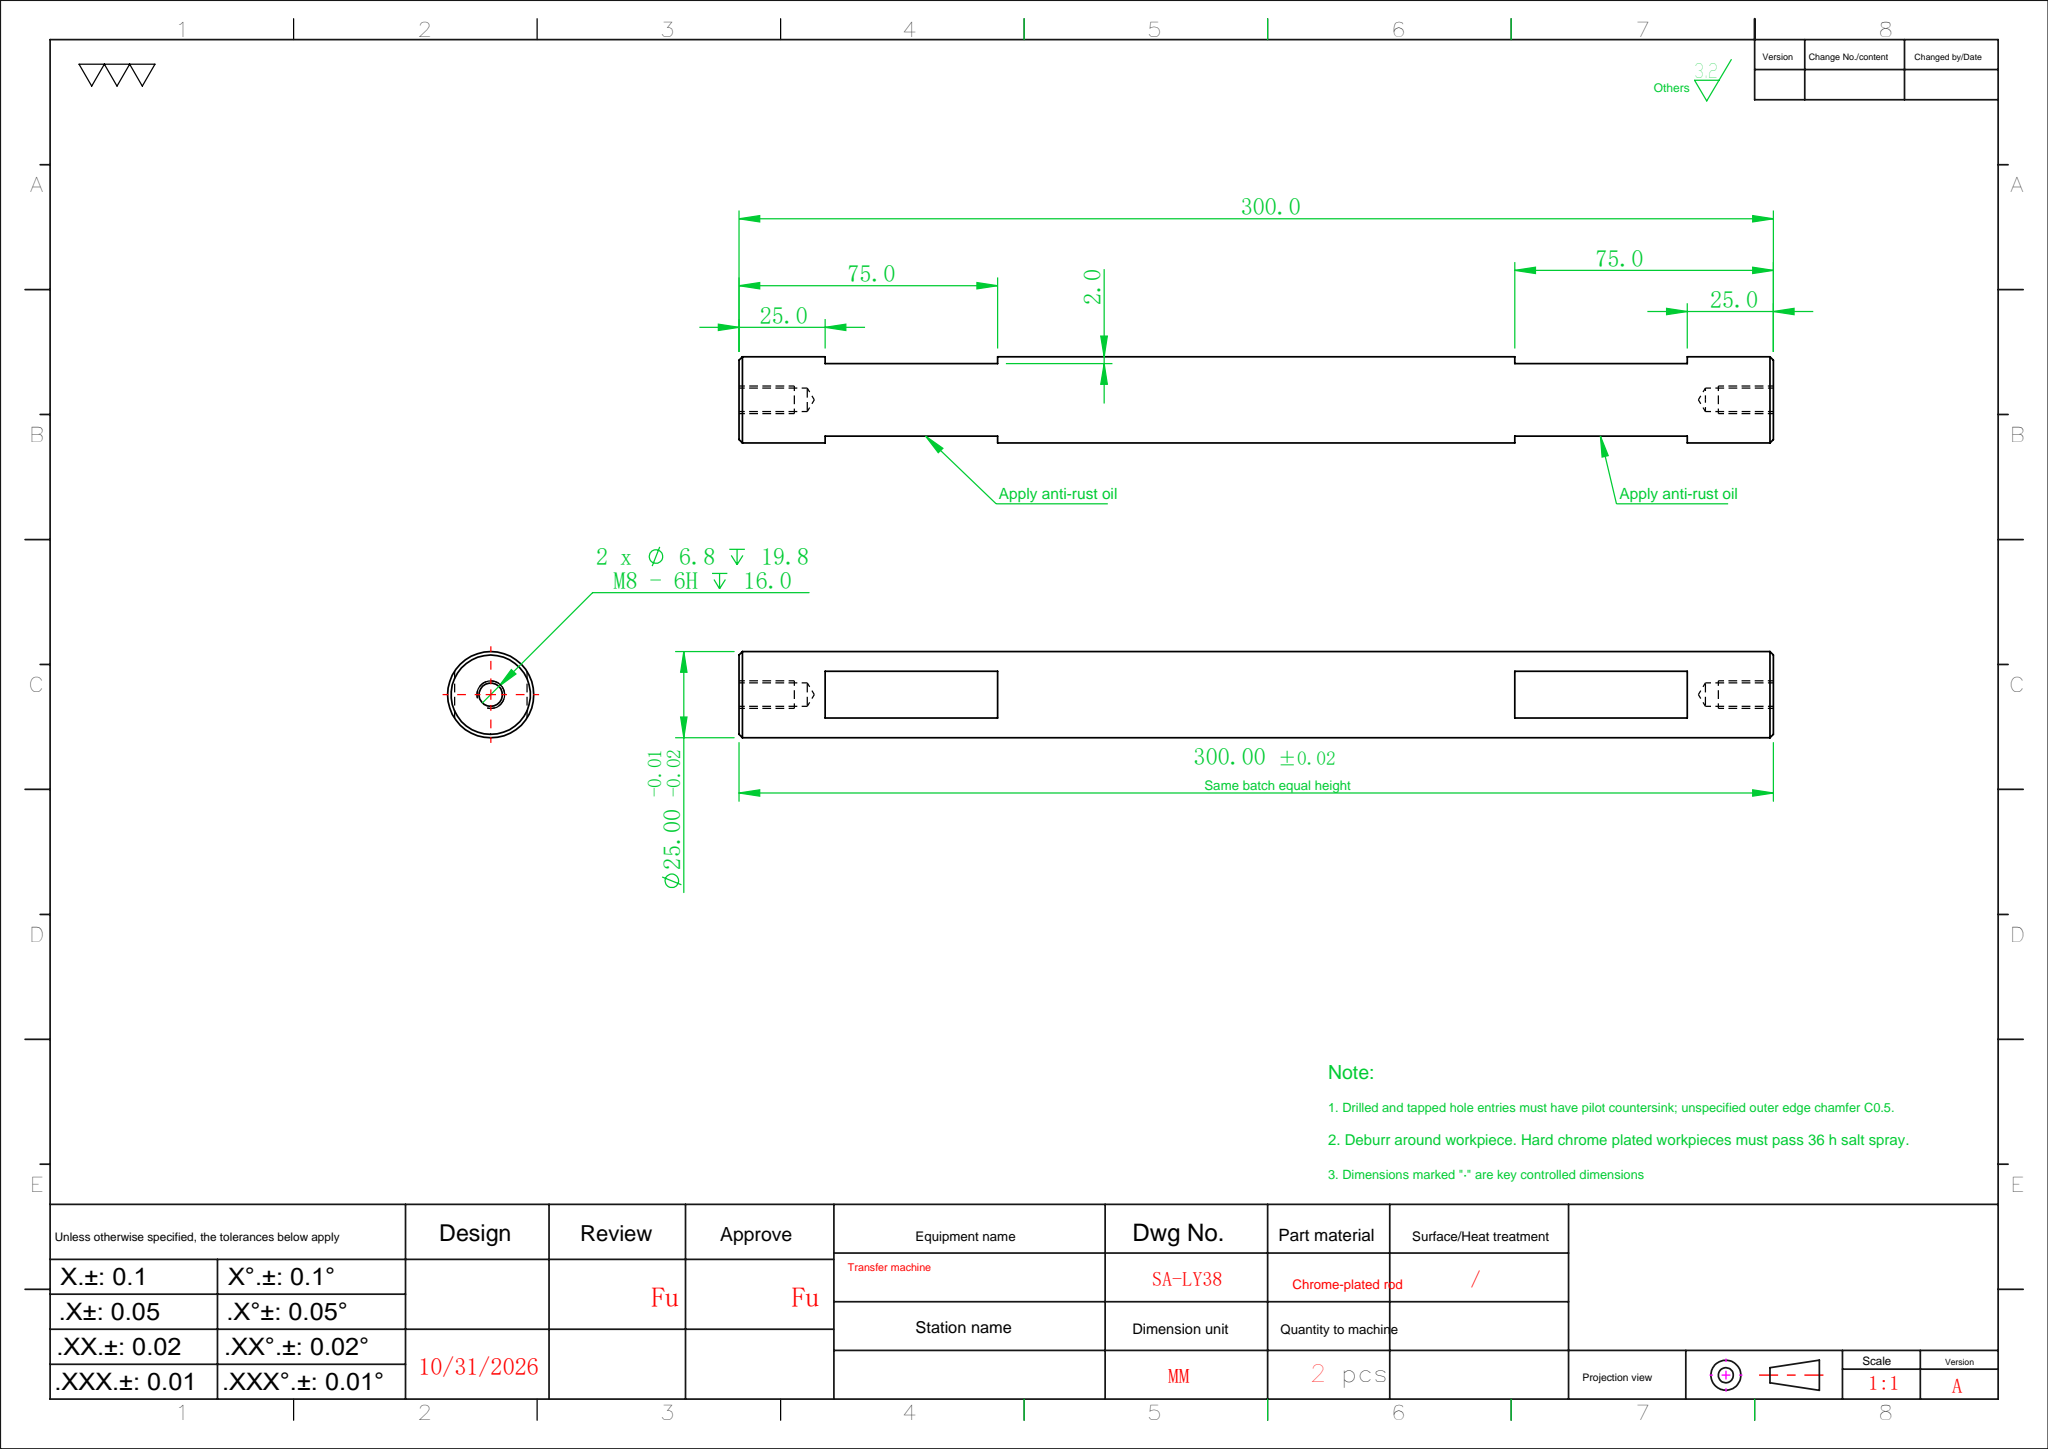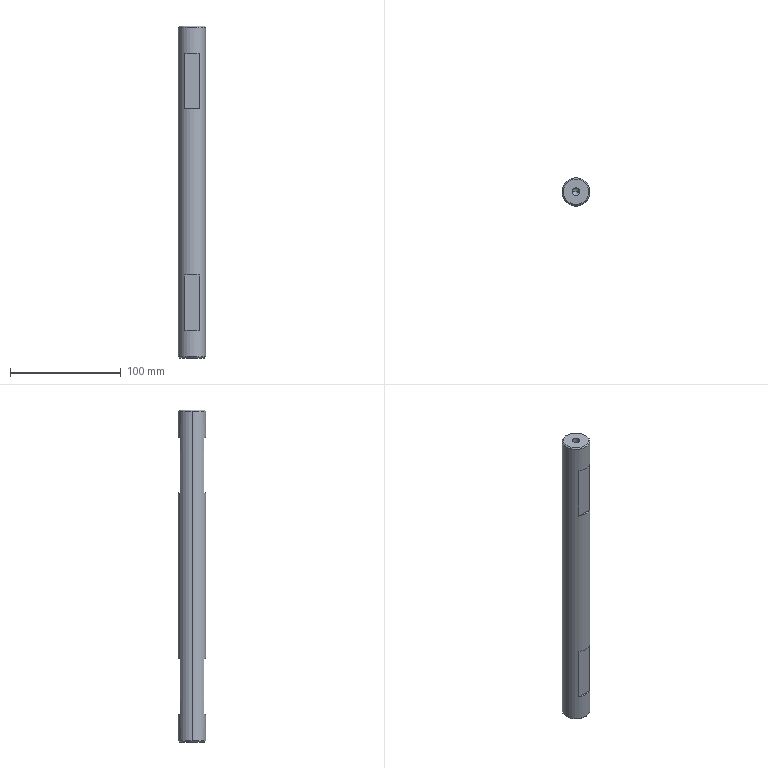Part | SolidWorks | features Chamfer 1, Extrusion 1, HoleWzd 1, ICE 1, MirrorPattern 1 | 1 solid | 28 faces | box 25 x 25 x 300 mm | volume 142022 mm3 | plane 14 | cone 8 | cylinder 6 | commonest cylinder face diameters 6.8 x4 25 x2
STEP:
#1=CARTESIAN_POINT('',(-3.4,0.,130.25));
#2=VERTEX_POINT('',#1);
#3=CARTESIAN_POINT('',(3.4,0.,130.25));
#4=VERTEX_POINT('',#3);
#5=CARTESIAN_POINT('',(0.,0.,130.25));
#6=DIRECTION('',(0.,0.,1.));
#7=DIRECTION('',(1.,0.,0.));
#8=AXIS2_PLACEMENT_3D('',#5,#6,#7);
#9=CIRCLE('',#8,3.4);
#10=EDGE_CURVE('',#2,#4,#9,.T.);
#11=ORIENTED_EDGE('',*,*,#10,.F.);
#12=CARTESIAN_POINT('',(-3.4,0.,150.));
#13=VERTEX_POINT('',#12);
#14=CARTESIAN_POINT('',(-3.4,0.,150.));
#15=DIRECTION('',(0.,0.,1.));
#16=VECTOR('',#15,1000.);
#17=LINE('',#14,#16);
#18=EDGE_CURVE('',#2,#13,#17,.T.);
#19=ORIENTED_EDGE('',*,*,#18,.T.);
#20=CARTESIAN_POINT('',(3.4,0.,150.));
#21=VERTEX_POINT('',#20);
#22=CARTESIAN_POINT('',(0.,0.,150.));
#23=DIRECTION('',(0.,0.,1.));
#24=DIRECTION('',(1.,0.,0.));
#25=AXIS2_PLACEMENT_3D('',#22,#23,#24);
#26=CIRCLE('',#25,3.4);
#27=EDGE_CURVE('',#13,#21,#26,.T.);
#28=ORIENTED_EDGE('',*,*,#27,.T.);
#29=CARTESIAN_POINT('',(3.4,0.,150.));
#30=DIRECTION('',(0.,0.,1.));
#31=VECTOR('',#30,1000.);
#32=LINE('',#29,#31);
#33=EDGE_CURVE('',#4,#21,#32,.T.);
#34=ORIENTED_EDGE('',*,*,#33,.F.);
#35=EDGE_LOOP('',(#11,#19,#28,#34));
#36=FACE_OUTER_BOUND('',#35,.T.);
#37=CARTESIAN_POINT('',(0.,0.,150.));
#38=DIRECTION('',(0.,0.,1.));
#39=DIRECTION('',(1.,0.,0.));
#40=AXIS2_PLACEMENT_3D('',#37,#38,#39);
#41=CYLINDRICAL_SURFACE('',#40,3.4);
#42=ADVANCED_FACE('',(#36),#41,.F.);
#43=CARTESIAN_POINT('',(0.,0.,128.207));
#44=VERTEX_POINT('',#43);
#45=CARTESIAN_POINT('',(3.4,0.,130.25));
#46=DIRECTION('',(0.8572,0.,0.515));
#47=VECTOR('',#46,1000.);
#48=LINE('',#45,#47);
#49=EDGE_CURVE('',#44,#4,#48,.T.);
#50=ORIENTED_EDGE('',*,*,#49,.F.);
#51=CARTESIAN_POINT('',(-3.4,0.,130.25));
#52=DIRECTION('',(-0.8572,0.,0.515));
#53=VECTOR('',#52,1000.);
#54=LINE('',#51,#53);
#55=EDGE_CURVE('',#44,#2,#54,.T.);
#56=ORIENTED_EDGE('',*,*,#55,.T.);
#57=ORIENTED_EDGE('',*,*,#10,.T.);
#58=EDGE_LOOP('',(#50,#56,#57));
#59=FACE_OUTER_BOUND('',#58,.T.);
#60=CARTESIAN_POINT('',(0.,0.,130.25));
#61=DIRECTION('',(0.,0.,1.));
#62=DIRECTION('',(1.,0.,0.));
#63=AXIS2_PLACEMENT_3D('',#60,#61,#62);
#64=CONICAL_SURFACE('',#63,3.4,1.03);
#65=ADVANCED_FACE('',(#59),#64,.F.);
#66=CARTESIAN_POINT('',(3.4,0.,-130.25));
#67=VERTEX_POINT('',#66);
#68=CARTESIAN_POINT('',(-3.4,0.,-130.25));
#69=VERTEX_POINT('',#68);
#70=CARTESIAN_POINT('',(0.,0.,-130.25));
#71=DIRECTION('',(0.,0.,-1.));
#72=DIRECTION('',(-1.,0.,0.));
#73=AXIS2_PLACEMENT_3D('',#70,#71,#72);
#74=CIRCLE('',#73,3.4);
#75=EDGE_CURVE('',#67,#69,#74,.T.);
#76=ORIENTED_EDGE('',*,*,#75,.F.);
#77=CARTESIAN_POINT('',(3.4,0.,-150.));
#78=VERTEX_POINT('',#77);
#79=CARTESIAN_POINT('',(3.4,0.,-150.));
#80=DIRECTION('',(0.,0.,-1.));
#81=VECTOR('',#80,1000.);
#82=LINE('',#79,#81);
#83=EDGE_CURVE('',#67,#78,#82,.T.);
#84=ORIENTED_EDGE('',*,*,#83,.T.);
#85=CARTESIAN_POINT('',(-3.4,0.,-150.));
#86=VERTEX_POINT('',#85);
#87=CARTESIAN_POINT('',(0.,0.,-150.));
#88=DIRECTION('',(0.,0.,-1.));
#89=DIRECTION('',(-1.,0.,0.));
#90=AXIS2_PLACEMENT_3D('',#87,#88,#89);
#91=CIRCLE('',#90,3.4);
#92=EDGE_CURVE('',#78,#86,#91,.T.);
#93=ORIENTED_EDGE('',*,*,#92,.T.);
#94=CARTESIAN_POINT('',(-3.4,0.,-150.));
#95=DIRECTION('',(0.,0.,-1.));
#96=VECTOR('',#95,1000.);
#97=LINE('',#94,#96);
#98=EDGE_CURVE('',#69,#86,#97,.T.);
#99=ORIENTED_EDGE('',*,*,#98,.F.);
#100=EDGE_LOOP('',(#76,#84,#93,#99));
#101=FACE_OUTER_BOUND('',#100,.T.);
#102=CARTESIAN_POINT('',(0.,0.,-150.));
#103=DIRECTION('',(0.,0.,-1.));
#104=DIRECTION('',(-1.,0.,0.));
#105=AXIS2_PLACEMENT_3D('',#102,#103,#104);
#106=CYLINDRICAL_SURFACE('',#105,3.4);
#107=ADVANCED_FACE('',(#101),#106,.F.);
#108=CARTESIAN_POINT('',(0.,0.,-128.207));
#109=VERTEX_POINT('',#108);
#110=CARTESIAN_POINT('',(-3.4,0.,-130.25));
#111=DIRECTION('',(-0.8572,0.,-0.515));
#112=VECTOR('',#111,1000.);
#113=LINE('',#110,#112);
#114=EDGE_CURVE('',#109,#69,#113,.T.);
#115=ORIENTED_EDGE('',*,*,#114,.F.);
#116=CARTESIAN_POINT('',(3.4,0.,-130.25));
#117=DIRECTION('',(0.8572,0.,-0.515));
#118=VECTOR('',#117,1000.);
#119=LINE('',#116,#118);
#120=EDGE_CURVE('',#109,#67,#119,.T.);
#121=ORIENTED_EDGE('',*,*,#120,.T.);
#122=ORIENTED_EDGE('',*,*,#75,.T.);
#123=EDGE_LOOP('',(#115,#121,#122));
#124=FACE_OUTER_BOUND('',#123,.T.);
#125=CARTESIAN_POINT('',(0.,0.,-130.25));
#126=DIRECTION('',(0.,0.,-1.));
#127=DIRECTION('',(-1.,0.,0.));
#128=AXIS2_PLACEMENT_3D('',#125,#126,#127);
#129=CONICAL_SURFACE('',#128,3.4,1.03);
#130=ADVANCED_FACE('',(#124),#129,.F.);
#131=CARTESIAN_POINT('',(-11.5,0.,-150.));
#132=VERTEX_POINT('',#131);
#133=CARTESIAN_POINT('',(11.5,0.,-150.));
#134=VERTEX_POINT('',#133);
#135=CARTESIAN_POINT('',(0.,0.,-150.));
#136=DIRECTION('',(0.,0.,-1.));
#137=DIRECTION('',(1.,0.,0.));
#138=AXIS2_PLACEMENT_3D('',#135,#136,#137);
#139=CIRCLE('',#138,11.5);
#140=EDGE_CURVE('',#132,#134,#139,.T.);
#141=ORIENTED_EDGE('',*,*,#140,.F.);
#142=CARTESIAN_POINT('',(-12.5,0.,-149.));
#143=VERTEX_POINT('',#142);
#144=CARTESIAN_POINT('',(-12.5,0.,-149.));
#145=DIRECTION('',(-0.7071,0.,0.7071));
#146=VECTOR('',#145,1000.);
#147=LINE('',#144,#146);
#148=EDGE_CURVE('',#132,#143,#147,.T.);
#149=ORIENTED_EDGE('',*,*,#148,.T.);
#150=CARTESIAN_POINT('',(12.5,0.,-149.));
#151=VERTEX_POINT('',#150);
#152=CARTESIAN_POINT('',(0.,0.,-149.));
#153=DIRECTION('',(0.,0.,1.));
#154=DIRECTION('',(1.,0.,0.));
#155=AXIS2_PLACEMENT_3D('',#152,#153,#154);
#156=CIRCLE('',#155,12.5);
#157=EDGE_CURVE('',#151,#143,#156,.T.);
#158=ORIENTED_EDGE('',*,*,#157,.F.);
#159=CARTESIAN_POINT('',(12.5,0.,-149.));
#160=DIRECTION('',(0.7071,0.,0.7071));
#161=VECTOR('',#160,1000.);
#162=LINE('',#159,#161);
#163=EDGE_CURVE('',#134,#151,#162,.T.);
#164=ORIENTED_EDGE('',*,*,#163,.F.);
#165=EDGE_LOOP('',(#141,#149,#158,#164));
#166=FACE_OUTER_BOUND('',#165,.T.);
#167=CARTESIAN_POINT('',(0.,0.,-149.));
#168=DIRECTION('',(0.,0.,1.));
#169=DIRECTION('',(1.,0.,0.));
#170=AXIS2_PLACEMENT_3D('',#167,#168,#169);
#171=CONICAL_SURFACE('',#170,12.5,0.7854);
#172=ADVANCED_FACE('',(#166),#171,.T.);
#173=CARTESIAN_POINT('',(11.5,0.,150.));
#174=VERTEX_POINT('',#173);
#175=CARTESIAN_POINT('',(-11.5,0.,150.));
#176=VERTEX_POINT('',#175);
#177=CARTESIAN_POINT('',(0.,0.,150.));
#178=DIRECTION('',(0.,0.,1.));
#179=DIRECTION('',(1.,0.,0.));
#180=AXIS2_PLACEMENT_3D('',#177,#178,#179);
#181=CIRCLE('',#180,11.5);
#182=EDGE_CURVE('',#174,#176,#181,.T.);
#183=ORIENTED_EDGE('',*,*,#182,.F.);
#184=CARTESIAN_POINT('',(12.5,0.,149.));
#185=VERTEX_POINT('',#184);
#186=CARTESIAN_POINT('',(11.5,0.,150.));
#187=DIRECTION('',(0.7071,0.,-0.7071));
#188=VECTOR('',#187,1000.);
#189=LINE('',#186,#188);
#190=EDGE_CURVE('',#174,#185,#189,.T.);
#191=ORIENTED_EDGE('',*,*,#190,.T.);
#192=CARTESIAN_POINT('',(-12.5,0.,149.));
#193=VERTEX_POINT('',#192);
#194=CARTESIAN_POINT('',(0.,0.,149.));
#195=DIRECTION('',(0.,0.,-1.));
#196=DIRECTION('',(1.,0.,0.));
#197=AXIS2_PLACEMENT_3D('',#194,#195,#196);
#198=CIRCLE('',#197,12.5);
#199=EDGE_CURVE('',#193,#185,#198,.T.);
#200=ORIENTED_EDGE('',*,*,#199,.F.);
#201=CARTESIAN_POINT('',(-11.5,0.,150.));
#202=DIRECTION('',(-0.7071,0.,-0.7071));
#203=VECTOR('',#202,1000.);
#204=LINE('',#201,#203);
#205=EDGE_CURVE('',#176,#193,#204,.T.);
#206=ORIENTED_EDGE('',*,*,#205,.F.);
#207=EDGE_LOOP('',(#183,#191,#200,#206));
#208=FACE_OUTER_BOUND('',#207,.T.);
#209=CARTESIAN_POINT('',(0.,0.,150.));
#210=DIRECTION('',(0.,0.,-1.));
#211=DIRECTION('',(-1.,0.,0.));
#212=AXIS2_PLACEMENT_3D('',#209,#210,#211);
#213=CONICAL_SURFACE('',#212,11.5,0.7854);
#214=ADVANCED_FACE('',(#208),#213,.T.);
#215=CARTESIAN_POINT('',(6.782,10.5,125.));
#216=VERTEX_POINT('',#215);
#217=CARTESIAN_POINT('',(-6.782,10.5,125.));
#218=VERTEX_POINT('',#217);
#219=CARTESIAN_POINT('',(0.,0.,125.));
#220=DIRECTION('',(0.,0.,1.));
#221=DIRECTION('',(1.,0.,0.));
#222=AXIS2_PLACEMENT_3D('',#219,#220,#221);
#223=CIRCLE('',#222,12.5);
#224=EDGE_CURVE('',#216,#218,#223,.T.);
#225=ORIENTED_EDGE('',*,*,#224,.T.);
#226=CARTESIAN_POINT('',(-6.782,10.5,75.));
#227=VERTEX_POINT('',#226);
#228=CARTESIAN_POINT('',(-6.782,10.5,150.));
#229=DIRECTION('',(0.,0.,-1.));
#230=VECTOR('',#229,1000.);
#231=LINE('',#228,#230);
#232=EDGE_CURVE('',#218,#227,#231,.T.);
#233=ORIENTED_EDGE('',*,*,#232,.T.);
#234=CARTESIAN_POINT('',(6.782,10.5,75.));
#235=VERTEX_POINT('',#234);
#236=CARTESIAN_POINT('',(0.,0.,75.));
#237=DIRECTION('',(0.,0.,-1.));
#238=DIRECTION('',(-1.,0.,0.));
#239=AXIS2_PLACEMENT_3D('',#236,#237,#238);
#240=CIRCLE('',#239,12.5);
#241=EDGE_CURVE('',#227,#235,#240,.T.);
#242=ORIENTED_EDGE('',*,*,#241,.T.);
#243=CARTESIAN_POINT('',(6.782,10.5,150.));
#244=DIRECTION('',(0.,0.,1.));
#245=VECTOR('',#244,1000.);
#246=LINE('',#243,#245);
#247=EDGE_CURVE('',#235,#216,#246,.T.);
#248=ORIENTED_EDGE('',*,*,#247,.T.);
#249=EDGE_LOOP('',(#225,#233,#242,#248));
#250=FACE_BOUND('',#249,.T.);
#251=CARTESIAN_POINT('',(-6.782,10.5,-75.));
#252=VERTEX_POINT('',#251);
#253=CARTESIAN_POINT('',(-6.782,10.5,-125.));
#254=VERTEX_POINT('',#253);
#255=CARTESIAN_POINT('',(-6.782,10.5,150.));
#256=DIRECTION('',(0.,0.,-1.));
#257=VECTOR('',#256,1000.);
#258=LINE('',#255,#257);
#259=EDGE_CURVE('',#252,#254,#258,.T.);
#260=ORIENTED_EDGE('',*,*,#259,.T.);
#261=CARTESIAN_POINT('',(6.782,10.5,-125.));
#262=VERTEX_POINT('',#261);
#263=CARTESIAN_POINT('',(0.,0.,-125.));
#264=DIRECTION('',(0.,0.,-1.));
#265=DIRECTION('',(-1.,0.,0.));
#266=AXIS2_PLACEMENT_3D('',#263,#264,#265);
#267=CIRCLE('',#266,12.5);
#268=EDGE_CURVE('',#254,#262,#267,.T.);
#269=ORIENTED_EDGE('',*,*,#268,.T.);
#270=CARTESIAN_POINT('',(6.782,10.5,-75.));
#271=VERTEX_POINT('',#270);
#272=CARTESIAN_POINT('',(6.782,10.5,150.));
#273=DIRECTION('',(0.,0.,1.));
#274=VECTOR('',#273,1000.);
#275=LINE('',#272,#274);
#276=EDGE_CURVE('',#262,#271,#275,.T.);
#277=ORIENTED_EDGE('',*,*,#276,.T.);
#278=CARTESIAN_POINT('',(0.,0.,-75.));
#279=DIRECTION('',(0.,0.,1.));
#280=DIRECTION('',(1.,0.,0.));
#281=AXIS2_PLACEMENT_3D('',#278,#279,#280);
#282=CIRCLE('',#281,12.5);
#283=EDGE_CURVE('',#271,#252,#282,.T.);
#284=ORIENTED_EDGE('',*,*,#283,.T.);
#285=EDGE_LOOP('',(#260,#269,#277,#284));
#286=FACE_BOUND('',#285,.T.);
#287=ORIENTED_EDGE('',*,*,#199,.T.);
#288=CARTESIAN_POINT('',(12.5,0.,150.));
#289=DIRECTION('',(0.,0.,-1.));
#290=VECTOR('',#289,1000.);
#291=LINE('',#288,#290);
#292=EDGE_CURVE('',#185,#151,#291,.T.);
#293=ORIENTED_EDGE('',*,*,#292,.T.);
#294=ORIENTED_EDGE('',*,*,#157,.T.);
#295=CARTESIAN_POINT('',(-12.5,0.,150.));
#296=DIRECTION('',(0.,0.,-1.));
#297=VECTOR('',#296,1000.);
#298=LINE('',#295,#297);
#299=EDGE_CURVE('',#193,#143,#298,.T.);
#300=ORIENTED_EDGE('',*,*,#299,.F.);
#301=EDGE_LOOP('',(#287,#293,#294,#300));
#302=FACE_OUTER_BOUND('',#301,.T.);
#303=CARTESIAN_POINT('',(0.,0.,150.));
#304=DIRECTION('',(0.,0.,-1.));
#305=DIRECTION('',(-1.,0.,0.));
#306=AXIS2_PLACEMENT_3D('',#303,#304,#305);
#307=CYLINDRICAL_SURFACE('',#306,12.5);
#308=ADVANCED_FACE('',(#250,#286,#302),#307,.T.);
#309=ORIENTED_EDGE('',*,*,#292,.F.);
#310=CARTESIAN_POINT('',(0.,0.,149.));
#311=DIRECTION('',(0.,0.,-1.));
#312=DIRECTION('',(1.,0.,0.));
#313=AXIS2_PLACEMENT_3D('',#310,#311,#312);
#314=CIRCLE('',#313,12.5);
#315=EDGE_CURVE('',#185,#193,#314,.T.);
#316=ORIENTED_EDGE('',*,*,#315,.T.);
#317=ORIENTED_EDGE('',*,*,#299,.T.);
#318=CARTESIAN_POINT('',(0.,0.,-149.));
#319=DIRECTION('',(0.,0.,1.));
#320=DIRECTION('',(1.,0.,0.));
#321=AXIS2_PLACEMENT_3D('',#318,#319,#320);
#322=CIRCLE('',#321,12.5);
#323=EDGE_CURVE('',#143,#151,#322,.T.);
#324=ORIENTED_EDGE('',*,*,#323,.T.);
#325=EDGE_LOOP('',(#309,#316,#317,#324));
#326=FACE_OUTER_BOUND('',#325,.T.);
#327=CARTESIAN_POINT('',(-6.782,-10.5,-75.));
#328=VERTEX_POINT('',#327);
#329=CARTESIAN_POINT('',(6.782,-10.5,-75.));
#330=VERTEX_POINT('',#329);
#331=CARTESIAN_POINT('',(0.,0.,-75.));
#332=DIRECTION('',(0.,0.,1.));
#333=DIRECTION('',(1.,0.,0.));
#334=AXIS2_PLACEMENT_3D('',#331,#332,#333);
#335=CIRCLE('',#334,12.5);
#336=EDGE_CURVE('',#328,#330,#335,.T.);
#337=ORIENTED_EDGE('',*,*,#336,.T.);
#338=CARTESIAN_POINT('',(6.782,-10.5,-125.));
#339=VERTEX_POINT('',#338);
#340=CARTESIAN_POINT('',(6.782,-10.5,150.));
#341=DIRECTION('',(0.,0.,-1.));
#342=VECTOR('',#341,1000.);
#343=LINE('',#340,#342);
#344=EDGE_CURVE('',#330,#339,#343,.T.);
#345=ORIENTED_EDGE('',*,*,#344,.T.);
#346=CARTESIAN_POINT('',(-6.782,-10.5,-125.));
#347=VERTEX_POINT('',#346);
#348=CARTESIAN_POINT('',(0.,0.,-125.));
#349=DIRECTION('',(0.,0.,-1.));
#350=DIRECTION('',(-1.,0.,0.));
#351=AXIS2_PLACEMENT_3D('',#348,#349,#350);
#352=CIRCLE('',#351,12.5);
#353=EDGE_CURVE('',#339,#347,#352,.T.);
#354=ORIENTED_EDGE('',*,*,#353,.T.);
#355=CARTESIAN_POINT('',(-6.782,-10.5,150.));
#356=DIRECTION('',(0.,0.,1.));
#357=VECTOR('',#356,1000.);
#358=LINE('',#355,#357);
#359=EDGE_CURVE('',#347,#328,#358,.T.);
#360=ORIENTED_EDGE('',*,*,#359,.T.);
#361=EDGE_LOOP('',(#337,#345,#354,#360));
#362=FACE_BOUND('',#361,.T.);
#363=CARTESIAN_POINT('',(-6.782,-10.5,75.));
#364=VERTEX_POINT('',#363);
#365=CARTESIAN_POINT('',(-6.782,-10.5,125.));
#366=VERTEX_POINT('',#365);
#367=CARTESIAN_POINT('',(-6.782,-10.5,150.));
#368=DIRECTION('',(0.,0.,1.));
#369=VECTOR('',#368,1000.);
#370=LINE('',#367,#369);
#371=EDGE_CURVE('',#364,#366,#370,.T.);
#372=ORIENTED_EDGE('',*,*,#371,.T.);
#373=CARTESIAN_POINT('',(6.782,-10.5,125.));
#374=VERTEX_POINT('',#373);
#375=CARTESIAN_POINT('',(0.,0.,125.));
#376=DIRECTION('',(0.,0.,1.));
#377=DIRECTION('',(1.,0.,0.));
#378=AXIS2_PLACEMENT_3D('',#375,#376,#377);
#379=CIRCLE('',#378,12.5);
#380=EDGE_CURVE('',#366,#374,#379,.T.);
#381=ORIENTED_EDGE('',*,*,#380,.T.);
#382=CARTESIAN_POINT('',(6.782,-10.5,75.));
#383=VERTEX_POINT('',#382);
#384=CARTESIAN_POINT('',(6.782,-10.5,150.));
#385=DIRECTION('',(0.,0.,-1.));
#386=VECTOR('',#385,1000.);
#387=LINE('',#384,#386);
#388=EDGE_CURVE('',#374,#383,#387,.T.);
#389=ORIENTED_EDGE('',*,*,#388,.T.);
#390=CARTESIAN_POINT('',(0.,0.,75.));
#391=DIRECTION('',(0.,0.,-1.));
#392=DIRECTION('',(-1.,0.,0.));
#393=AXIS2_PLACEMENT_3D('',#390,#391,#392);
#394=CIRCLE('',#393,12.5);
#395=EDGE_CURVE('',#383,#364,#394,.T.);
#396=ORIENTED_EDGE('',*,*,#395,.T.);
#397=EDGE_LOOP('',(#372,#381,#389,#396));
#398=FACE_BOUND('',#397,.T.);
#399=CARTESIAN_POINT('',(0.,0.,150.));
#400=DIRECTION('',(0.,0.,-1.));
#401=DIRECTION('',(-1.,0.,0.));
#402=AXIS2_PLACEMENT_3D('',#399,#400,#401);
#403=CYLINDRICAL_SURFACE('',#402,12.5);
#404=ADVANCED_FACE('',(#326,#362,#398),#403,.T.);
#405=CARTESIAN_POINT('',(0.,0.,150.));
#406=DIRECTION('',(0.,0.,1.));
#407=DIRECTION('',(1.,0.,0.));
#408=AXIS2_PLACEMENT_3D('',#405,#406,#407);
#409=CIRCLE('',#408,3.4);
#410=EDGE_CURVE('',#21,#13,#409,.T.);
#411=ORIENTED_EDGE('',*,*,#410,.F.);
#412=ORIENTED_EDGE('',*,*,#27,.F.);
#413=EDGE_LOOP('',(#411,#412));
#414=FACE_BOUND('',#413,.T.);
#415=CARTESIAN_POINT('',(0.,0.,150.));
#416=DIRECTION('',(0.,0.,1.));
#417=DIRECTION('',(1.,0.,0.));
#418=AXIS2_PLACEMENT_3D('',#415,#416,#417);
#419=CIRCLE('',#418,11.5);
#420=EDGE_CURVE('',#176,#174,#419,.T.);
#421=ORIENTED_EDGE('',*,*,#420,.T.);
#422=ORIENTED_EDGE('',*,*,#182,.T.);
#423=EDGE_LOOP('',(#421,#422));
#424=FACE_OUTER_BOUND('',#423,.T.);
#425=CARTESIAN_POINT('',(0.,0.,150.));
#426=DIRECTION('',(0.,0.,1.));
#427=DIRECTION('',(1.,0.,0.));
#428=AXIS2_PLACEMENT_3D('',#425,#426,#427);
#429=PLANE('',#428);
#430=ADVANCED_FACE('',(#414,#424),#429,.T.);
#431=CARTESIAN_POINT('',(0.,0.,-150.));
#432=DIRECTION('',(0.,0.,-1.));
#433=DIRECTION('',(-1.,0.,0.));
#434=AXIS2_PLACEMENT_3D('',#431,#432,#433);
#435=CIRCLE('',#434,3.4);
#436=EDGE_CURVE('',#86,#78,#435,.T.);
#437=ORIENTED_EDGE('',*,*,#436,.F.);
#438=ORIENTED_EDGE('',*,*,#92,.F.);
#439=EDGE_LOOP('',(#437,#438));
#440=FACE_BOUND('',#439,.T.);
#441=CARTESIAN_POINT('',(0.,0.,-150.));
#442=DIRECTION('',(0.,0.,-1.));
#443=DIRECTION('',(1.,0.,0.));
#444=AXIS2_PLACEMENT_3D('',#441,#442,#443);
#445=CIRCLE('',#444,11.5);
#446=EDGE_CURVE('',#134,#132,#445,.T.);
#447=ORIENTED_EDGE('',*,*,#446,.T.);
#448=ORIENTED_EDGE('',*,*,#140,.T.);
#449=EDGE_LOOP('',(#447,#448));
#450=FACE_OUTER_BOUND('',#449,.T.);
#451=CARTESIAN_POINT('',(0.,0.,-150.));
#452=DIRECTION('',(0.,0.,1.));
#453=DIRECTION('',(1.,0.,0.));
#454=AXIS2_PLACEMENT_3D('',#451,#452,#453);
#455=PLANE('',#454);
#456=ADVANCED_FACE('',(#440,#450),#455,.F.);
#457=CARTESIAN_POINT('',(-100.,10.5,125.));
#458=DIRECTION('',(1.,0.,0.));
#459=VECTOR('',#458,1000.);
#460=LINE('',#457,#459);
#461=EDGE_CURVE('',#218,#216,#460,.T.);
#462=ORIENTED_EDGE('',*,*,#461,.F.);
#463=ORIENTED_EDGE('',*,*,#224,.F.);
#464=EDGE_LOOP('',(#462,#463));
#465=FACE_OUTER_BOUND('',#464,.T.);
#466=CARTESIAN_POINT('',(-100.,12.5,125.));
#467=DIRECTION('',(0.,0.,1.));
#468=DIRECTION('',(1.,0.,0.));
#469=AXIS2_PLACEMENT_3D('',#466,#467,#468);
#470=PLANE('',#469);
#471=ADVANCED_FACE('',(#465),#470,.F.);
#472=CARTESIAN_POINT('',(-100.,10.5,75.));
#473=DIRECTION('',(1.,0.,0.));
#474=VECTOR('',#473,1000.);
#475=LINE('',#472,#474);
#476=EDGE_CURVE('',#227,#235,#475,.T.);
#477=ORIENTED_EDGE('',*,*,#476,.T.);
#478=ORIENTED_EDGE('',*,*,#241,.F.);
#479=EDGE_LOOP('',(#477,#478));
#480=FACE_OUTER_BOUND('',#479,.T.);
#481=CARTESIAN_POINT('',(-100.,12.5,75.));
#482=DIRECTION('',(0.,0.,-1.));
#483=DIRECTION('',(-1.,0.,0.));
#484=AXIS2_PLACEMENT_3D('',#481,#482,#483);
#485=PLANE('',#484);
#486=ADVANCED_FACE('',(#480),#485,.F.);
#487=ORIENTED_EDGE('',*,*,#461,.T.);
#488=ORIENTED_EDGE('',*,*,#247,.F.);
#489=ORIENTED_EDGE('',*,*,#476,.F.);
#490=ORIENTED_EDGE('',*,*,#232,.F.);
#491=EDGE_LOOP('',(#487,#488,#489,#490));
#492=FACE_OUTER_BOUND('',#491,.T.);
#493=CARTESIAN_POINT('',(-100.,10.5,125.));
#494=DIRECTION('',(0.,-1.,0.));
#495=DIRECTION('',(0.,0.,-1.));
#496=AXIS2_PLACEMENT_3D('',#493,#494,#495);
#497=PLANE('',#496);
#498=ADVANCED_FACE('',(#492),#497,.F.);
#499=CARTESIAN_POINT('',(-100.,-10.5,125.));
#500=DIRECTION('',(1.,0.,0.));
#501=VECTOR('',#500,1000.);
#502=LINE('',#499,#501);
#503=EDGE_CURVE('',#366,#374,#502,.T.);
#504=ORIENTED_EDGE('',*,*,#503,.T.);
#505=ORIENTED_EDGE('',*,*,#380,.F.);
#506=EDGE_LOOP('',(#504,#505));
#507=FACE_OUTER_BOUND('',#506,.T.);
#508=CARTESIAN_POINT('',(-100.,-12.5,125.));
#509=DIRECTION('',(0.,0.,1.));
#510=DIRECTION('',(1.,0.,0.));
#511=AXIS2_PLACEMENT_3D('',#508,#509,#510);
#512=PLANE('',#511);
#513=ADVANCED_FACE('',(#507),#512,.F.);
#514=ORIENTED_EDGE('',*,*,#503,.F.);
#515=ORIENTED_EDGE('',*,*,#371,.F.);
#516=CARTESIAN_POINT('',(-100.,-10.5,75.));
#517=DIRECTION('',(1.,0.,0.));
#518=VECTOR('',#517,1000.);
#519=LINE('',#516,#518);
#520=EDGE_CURVE('',#364,#383,#519,.T.);
#521=ORIENTED_EDGE('',*,*,#520,.T.);
#522=ORIENTED_EDGE('',*,*,#388,.F.);
#523=EDGE_LOOP('',(#514,#515,#521,#522));
#524=FACE_OUTER_BOUND('',#523,.T.);
#525=CARTESIAN_POINT('',(-100.,-10.5,125.));
#526=DIRECTION('',(0.,1.,0.));
#527=DIRECTION('',(0.,0.,1.));
#528=AXIS2_PLACEMENT_3D('',#525,#526,#527);
#529=PLANE('',#528);
#530=ADVANCED_FACE('',(#524),#529,.F.);
#531=ORIENTED_EDGE('',*,*,#520,.F.);
#532=ORIENTED_EDGE('',*,*,#395,.F.);
#533=EDGE_LOOP('',(#531,#532));
#534=FACE_OUTER_BOUND('',#533,.T.);
#535=CARTESIAN_POINT('',(-100.,-12.5,75.));
#536=DIRECTION('',(0.,0.,-1.));
#537=DIRECTION('',(-1.,0.,0.));
#538=AXIS2_PLACEMENT_3D('',#535,#536,#537);
#539=PLANE('',#538);
#540=ADVANCED_FACE('',(#534),#539,.F.);
#541=CARTESIAN_POINT('',(-100.,-10.5,-125.));
#542=DIRECTION('',(1.,0.,0.));
#543=VECTOR('',#542,1000.);
#544=LINE('',#541,#543);
#545=EDGE_CURVE('',#347,#339,#544,.T.);
#546=ORIENTED_EDGE('',*,*,#545,.F.);
#547=ORIENTED_EDGE('',*,*,#353,.F.);
#548=EDGE_LOOP('',(#546,#547));
#549=FACE_OUTER_BOUND('',#548,.T.);
#550=CARTESIAN_POINT('',(-100.,-12.5,-125.));
#551=DIRECTION('',(0.,0.,-1.));
#552=DIRECTION('',(-1.,0.,0.));
#553=AXIS2_PLACEMENT_3D('',#550,#551,#552);
#554=PLANE('',#553);
#555=ADVANCED_FACE('',(#549),#554,.F.);
#556=CARTESIAN_POINT('',(-100.,-10.5,-75.));
#557=DIRECTION('',(1.,0.,0.));
#558=VECTOR('',#557,1000.);
#559=LINE('',#556,#558);
#560=EDGE_CURVE('',#328,#330,#559,.T.);
#561=ORIENTED_EDGE('',*,*,#560,.T.);
#562=ORIENTED_EDGE('',*,*,#336,.F.);
#563=EDGE_LOOP('',(#561,#562));
#564=FACE_OUTER_BOUND('',#563,.T.);
#565=CARTESIAN_POINT('',(-100.,-12.5,-75.));
#566=DIRECTION('',(0.,0.,1.));
#567=DIRECTION('',(1.,0.,0.));
#568=AXIS2_PLACEMENT_3D('',#565,#566,#567);
#569=PLANE('',#568);
#570=ADVANCED_FACE('',(#564),#569,.F.);
#571=ORIENTED_EDGE('',*,*,#560,.F.);
#572=ORIENTED_EDGE('',*,*,#359,.F.);
#573=ORIENTED_EDGE('',*,*,#545,.T.);
#574=ORIENTED_EDGE('',*,*,#344,.F.);
#575=EDGE_LOOP('',(#571,#572,#573,#574));
#576=FACE_OUTER_BOUND('',#575,.T.);
#577=CARTESIAN_POINT('',(-100.,-10.5,-125.));
#578=DIRECTION('',(0.,1.,0.));
#579=DIRECTION('',(0.,0.,1.));
#580=AXIS2_PLACEMENT_3D('',#577,#578,#579);
#581=PLANE('',#580);
#582=ADVANCED_FACE('',(#576),#581,.F.);
#583=CARTESIAN_POINT('',(-100.,10.5,-125.));
#584=DIRECTION('',(1.,0.,0.));
#585=VECTOR('',#584,1000.);
#586=LINE('',#583,#585);
#587=EDGE_CURVE('',#254,#262,#586,.T.);
#588=ORIENTED_EDGE('',*,*,#587,.T.);
#589=ORIENTED_EDGE('',*,*,#268,.F.);
#590=EDGE_LOOP('',(#588,#589));
#591=FACE_OUTER_BOUND('',#590,.T.);
#592=CARTESIAN_POINT('',(-100.,12.5,-125.));
#593=DIRECTION('',(0.,0.,-1.));
#594=DIRECTION('',(-1.,0.,0.));
#595=AXIS2_PLACEMENT_3D('',#592,#593,#594);
#596=PLANE('',#595);
#597=ADVANCED_FACE('',(#591),#596,.F.);
#598=CARTESIAN_POINT('',(-100.,10.5,-75.));
#599=DIRECTION('',(1.,0.,0.));
#600=VECTOR('',#599,1000.);
#601=LINE('',#598,#600);
#602=EDGE_CURVE('',#252,#271,#601,.T.);
#603=ORIENTED_EDGE('',*,*,#602,.T.);
#604=ORIENTED_EDGE('',*,*,#276,.F.);
#605=ORIENTED_EDGE('',*,*,#587,.F.);
#606=ORIENTED_EDGE('',*,*,#259,.F.);
#607=EDGE_LOOP('',(#603,#604,#605,#606));
#608=FACE_OUTER_BOUND('',#607,.T.);
#609=CARTESIAN_POINT('',(-100.,10.5,-125.));
#610=DIRECTION('',(0.,-1.,0.));
#611=DIRECTION('',(0.,0.,-1.));
#612=AXIS2_PLACEMENT_3D('',#609,#610,#611);
#613=PLANE('',#612);
#614=ADVANCED_FACE('',(#608),#613,.F.);
#615=ORIENTED_EDGE('',*,*,#602,.F.);
#616=ORIENTED_EDGE('',*,*,#283,.F.);
#617=EDGE_LOOP('',(#615,#616));
#618=FACE_OUTER_BOUND('',#617,.T.);
#619=CARTESIAN_POINT('',(-100.,12.5,-75.));
#620=DIRECTION('',(0.,0.,1.));
#621=DIRECTION('',(1.,0.,0.));
#622=AXIS2_PLACEMENT_3D('',#619,#620,#621);
#623=PLANE('',#622);
#624=ADVANCED_FACE('',(#618),#623,.F.);
#625=ORIENTED_EDGE('',*,*,#190,.F.);
#626=ORIENTED_EDGE('',*,*,#420,.F.);
#627=ORIENTED_EDGE('',*,*,#205,.T.);
#628=ORIENTED_EDGE('',*,*,#315,.F.);
#629=EDGE_LOOP('',(#625,#626,#627,#628));
#630=FACE_OUTER_BOUND('',#629,.T.);
#631=CARTESIAN_POINT('',(0.,0.,150.));
#632=DIRECTION('',(0.,0.,-1.));
#633=DIRECTION('',(-1.,0.,0.));
#634=AXIS2_PLACEMENT_3D('',#631,#632,#633);
#635=CONICAL_SURFACE('',#634,11.5,0.7854);
#636=ADVANCED_FACE('',(#630),#635,.T.);
#637=ORIENTED_EDGE('',*,*,#148,.F.);
#638=ORIENTED_EDGE('',*,*,#446,.F.);
#639=ORIENTED_EDGE('',*,*,#163,.T.);
#640=ORIENTED_EDGE('',*,*,#323,.F.);
#641=EDGE_LOOP('',(#637,#638,#639,#640));
#642=FACE_OUTER_BOUND('',#641,.T.);
#643=CARTESIAN_POINT('',(0.,0.,-149.));
#644=DIRECTION('',(0.,0.,1.));
#645=DIRECTION('',(1.,0.,0.));
#646=AXIS2_PLACEMENT_3D('',#643,#644,#645);
#647=CONICAL_SURFACE('',#646,12.5,0.7854);
#648=ADVANCED_FACE('',(#642),#647,.T.);
#649=ORIENTED_EDGE('',*,*,#120,.F.);
#650=ORIENTED_EDGE('',*,*,#114,.T.);
#651=CARTESIAN_POINT('',(0.,0.,-130.25));
#652=DIRECTION('',(0.,0.,-1.));
#653=DIRECTION('',(-1.,0.,0.));
#654=AXIS2_PLACEMENT_3D('',#651,#652,#653);
#655=CIRCLE('',#654,3.4);
#656=EDGE_CURVE('',#69,#67,#655,.T.);
#657=ORIENTED_EDGE('',*,*,#656,.T.);
#658=EDGE_LOOP('',(#649,#650,#657));
#659=FACE_OUTER_BOUND('',#658,.T.);
#660=CARTESIAN_POINT('',(0.,0.,-130.25));
#661=DIRECTION('',(0.,0.,-1.));
#662=DIRECTION('',(-1.,0.,0.));
#663=AXIS2_PLACEMENT_3D('',#660,#661,#662);
#664=CONICAL_SURFACE('',#663,3.4,1.03);
#665=ADVANCED_FACE('',(#659),#664,.F.);
#666=ORIENTED_EDGE('',*,*,#83,.F.);
#667=ORIENTED_EDGE('',*,*,#656,.F.);
#668=ORIENTED_EDGE('',*,*,#98,.T.);
#669=ORIENTED_EDGE('',*,*,#436,.T.);
#670=EDGE_LOOP('',(#666,#667,#668,#669));
#671=FACE_OUTER_BOUND('',#670,.T.);
#672=CARTESIAN_POINT('',(0.,0.,-150.));
#673=DIRECTION('',(0.,0.,-1.));
#674=DIRECTION('',(-1.,0.,0.));
#675=AXIS2_PLACEMENT_3D('',#672,#673,#674);
#676=CYLINDRICAL_SURFACE('',#675,3.4);
#677=ADVANCED_FACE('',(#671),#676,.F.);
#678=ORIENTED_EDGE('',*,*,#55,.F.);
#679=ORIENTED_EDGE('',*,*,#49,.T.);
#680=CARTESIAN_POINT('',(0.,0.,130.25));
#681=DIRECTION('',(0.,0.,1.));
#682=DIRECTION('',(1.,0.,0.));
#683=AXIS2_PLACEMENT_3D('',#680,#681,#682);
#684=CIRCLE('',#683,3.4);
#685=EDGE_CURVE('',#4,#2,#684,.T.);
#686=ORIENTED_EDGE('',*,*,#685,.T.);
#687=EDGE_LOOP('',(#678,#679,#686));
#688=FACE_OUTER_BOUND('',#687,.T.);
#689=CARTESIAN_POINT('',(0.,0.,130.25));
#690=DIRECTION('',(0.,0.,1.));
#691=DIRECTION('',(1.,0.,0.));
#692=AXIS2_PLACEMENT_3D('',#689,#690,#691);
#693=CONICAL_SURFACE('',#692,3.4,1.03);
#694=ADVANCED_FACE('',(#688),#693,.F.);
#695=ORIENTED_EDGE('',*,*,#18,.F.);
#696=ORIENTED_EDGE('',*,*,#685,.F.);
#697=ORIENTED_EDGE('',*,*,#33,.T.);
#698=ORIENTED_EDGE('',*,*,#410,.T.);
#699=EDGE_LOOP('',(#695,#696,#697,#698));
#700=FACE_OUTER_BOUND('',#699,.T.);
#701=CARTESIAN_POINT('',(0.,0.,150.));
#702=DIRECTION('',(0.,0.,1.));
#703=DIRECTION('',(1.,0.,0.));
#704=AXIS2_PLACEMENT_3D('',#701,#702,#703);
#705=CYLINDRICAL_SURFACE('',#704,3.4);
#706=ADVANCED_FACE('',(#700),#705,.F.);
#707=CLOSED_SHELL('',(#42,#65,#107,#130,#172,#214,#308,#404,#430,#456,#471,#486,#498,#513,#530,#540,#555,#570,#582,#597,#614,#624,#636,#648,#665,#677,#694,#706));
#708=MANIFOLD_SOLID_BREP('',#707);
#709=CARTESIAN_POINT('',(0.,0.,0.));
#710=DIRECTION('',(0.,0.,1.));
#711=DIRECTION('',(1.,0.,0.));
#712=AXIS2_PLACEMENT_3D('',#709,#710,#711);
#713=(LENGTH_UNIT()NAMED_UNIT(*)SI_UNIT(.MILLI.,.METRE.));
#714=UNCERTAINTY_MEASURE_WITH_UNIT(LENGTH_MEASURE(0.00001),#713,'','');
#715=(NAMED_UNIT(*)PLANE_ANGLE_UNIT()SI_UNIT($,.RADIAN.));
#716=(NAMED_UNIT(*)SI_UNIT($,.STERADIAN.)SOLID_ANGLE_UNIT());
#717=(GEOMETRIC_REPRESENTATION_CONTEXT(3)GLOBAL_UNCERTAINTY_ASSIGNED_CONTEXT((#714))GLOBAL_UNIT_ASSIGNED_CONTEXT((#713,#715,#716))REPRESENTATION_CONTEXT('',''));
#718=ADVANCED_BREP_SHAPE_REPRESENTATION('',(#708,#712),#717);